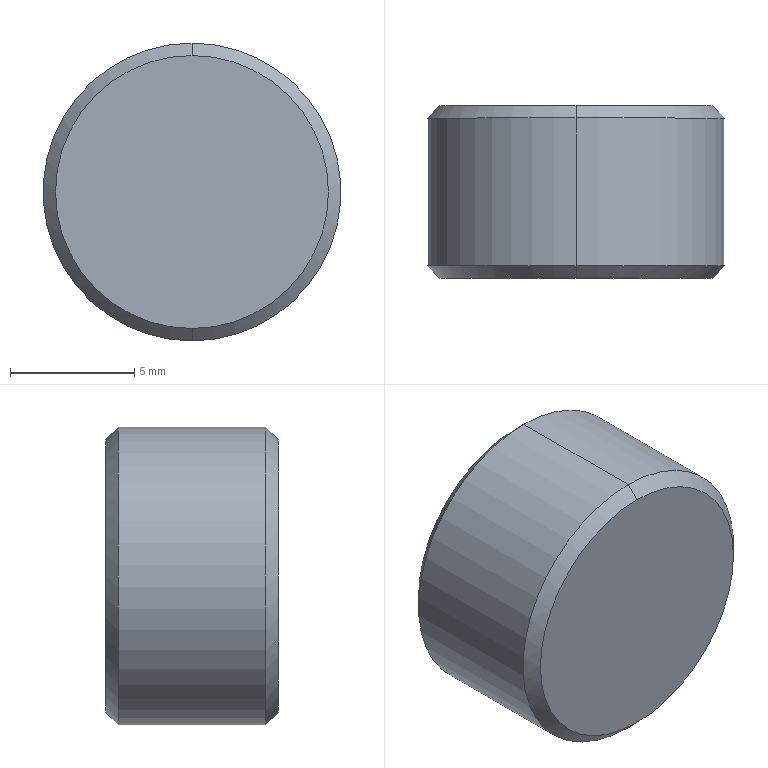Part | STEP file | 1-4 plug | 1 solid | 17 faces | box 12 x 6.95 x 12 mm | volume 518.038 mm3 | plane 9 | cone 6 | cylinder 2 | commonest cylinder face diameters 12 x2